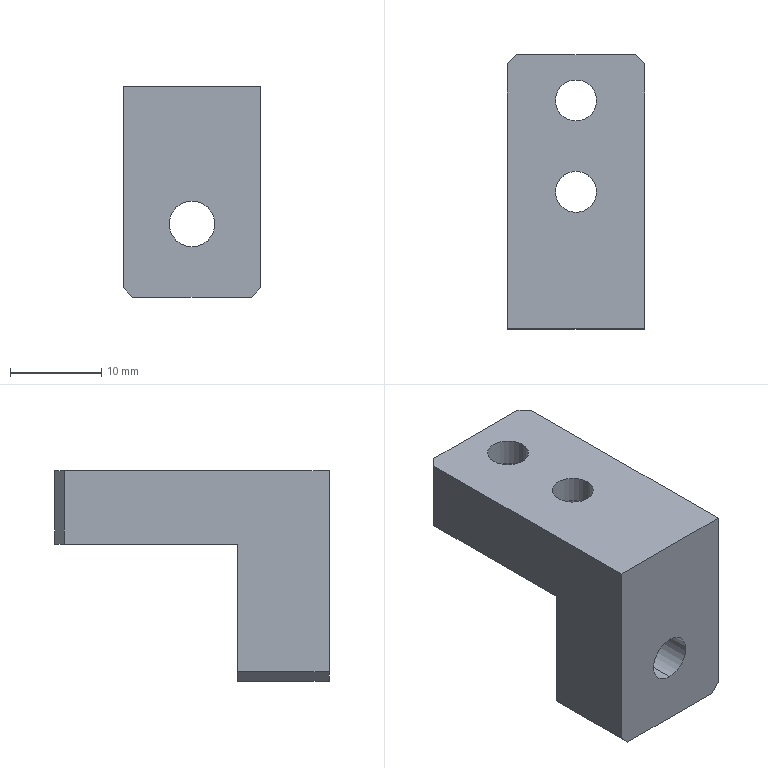Part | STEP file | 227H056261 Stop Block_Default | 1 solid | 24 faces | box 15 x 30 x 23 mm | volume 5038 mm3 | plane 14 | cylinder 10 | commonest cylinder face diameters 4.5 x4 8 x4 5 x2